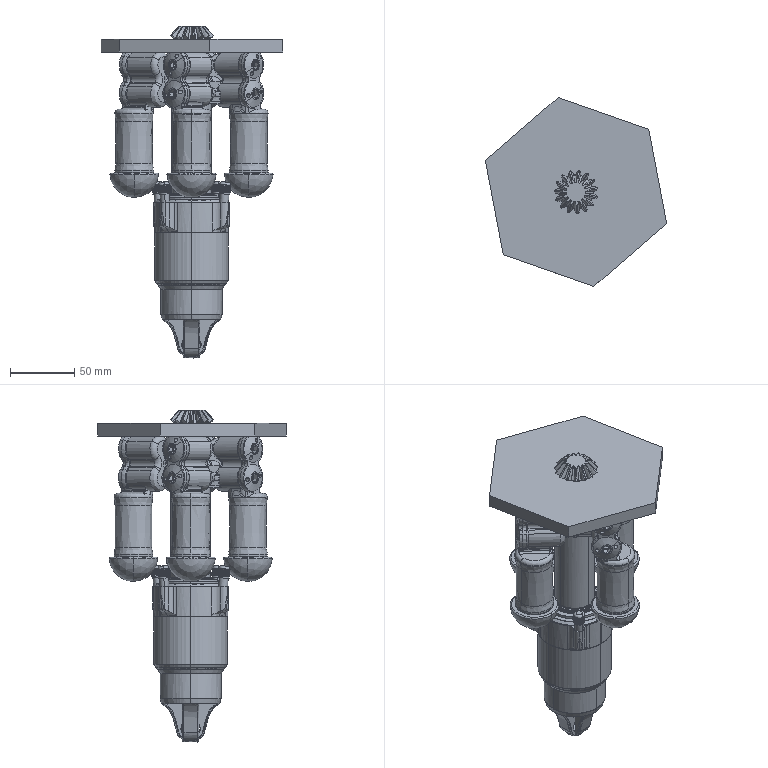Part | SolidWorks | 29 solids | 2990 faces | box 141.618 x 147.365 x 259.286 mm | volume 1445767 mm3 | plane 1400 | spline 613 | cylinder 498 | torus 252 | cone 211 | sphere 16 | commonest cylinder face diameters 0.483 x64 2 x40 3 x32 14.718 x24 21 x24 23.2 x24